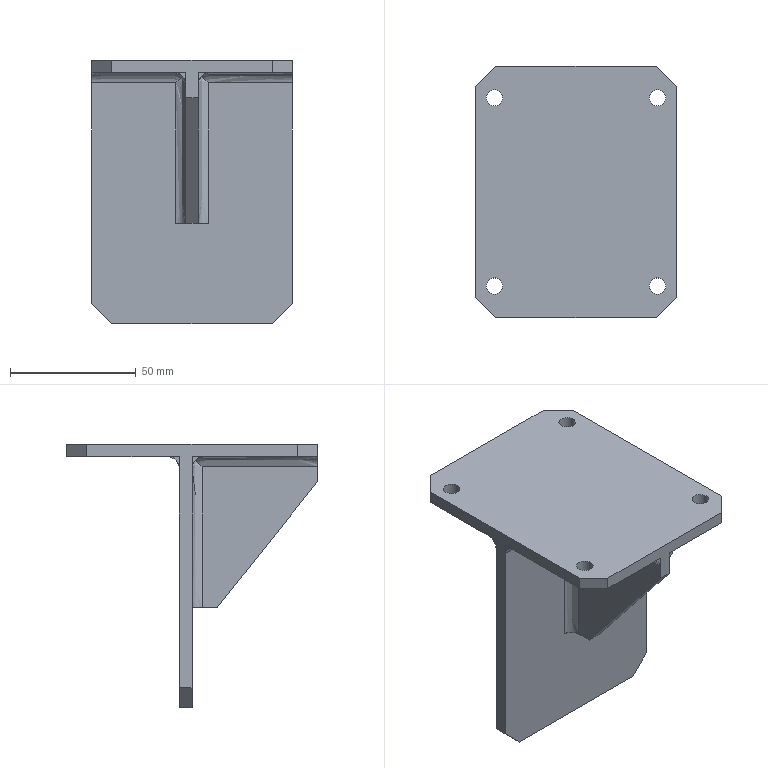Part | NX | features FILLET_WELD 5, FSET 5, EXTRUDE 3, DATUM_CSYS 2, UNITE 2, CHAMFER 1, SKETCH 1 | 4 solids | 48 faces | box 80 x 100 x 105 mm | volume 89889 mm3 | plane 37 | spline 7 | cylinder 4 | commonest cylinder face diameters 6.5 x4